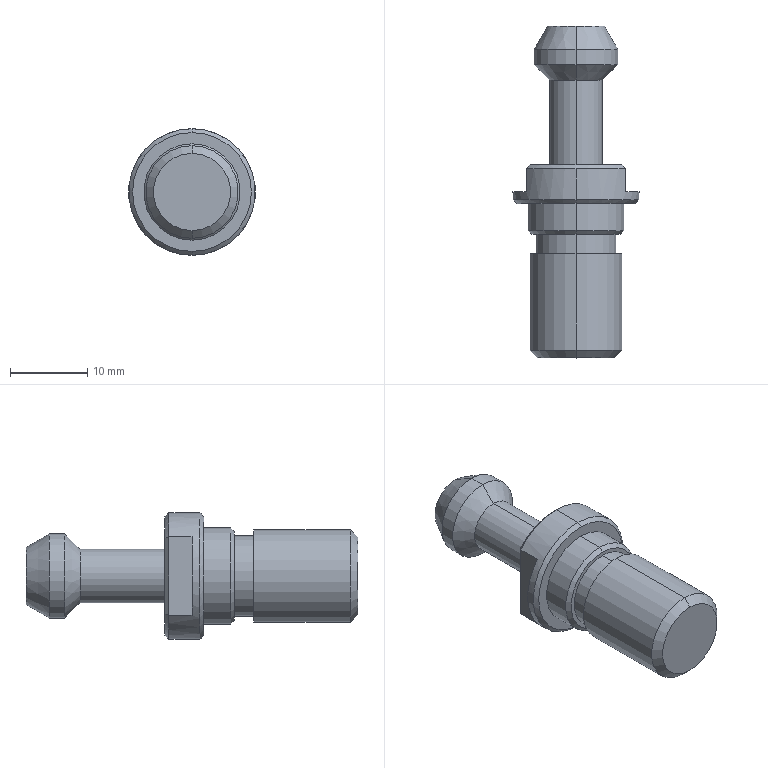Part | SolidWorks | features Chamfer 2, ICE 1, Revolution 1 | 1 solid | 37 faces | box 16.4 x 43 x 16.4 mm | volume 4091 mm3 | cone 13 | cylinder 12 | plane 12 | commonest cylinder face diameters 6.9 x2 10.4 x2 10.9 x2 12 x2 12.5 x2 16.4 x2
STEP:
#1=CARTESIAN_POINT('',(0.,16.,-5.75));
#2=VERTEX_POINT('',#1);
#3=CARTESIAN_POINT('',(0.,16.,5.75));
#4=VERTEX_POINT('',#3);
#5=CARTESIAN_POINT('',(0.,16.,0.));
#6=DIRECTION('',(0.,-1.,0.));
#7=DIRECTION('',(0.,0.,-1.));
#8=AXIS2_PLACEMENT_3D('',#5,#6,#7);
#9=CIRCLE('',#8,5.75);
#10=EDGE_CURVE('',#2,#4,#9,.T.);
#11=ORIENTED_EDGE('',*,*,#10,.F.);
#12=CARTESIAN_POINT('',(0.,16.5,-6.25));
#13=VERTEX_POINT('',#12);
#14=CARTESIAN_POINT('',(0.,16.,-5.75));
#15=DIRECTION('',(0.,0.7071,-0.7071));
#16=VECTOR('',#15,1000.);
#17=LINE('',#14,#16);
#18=EDGE_CURVE('',#2,#13,#17,.T.);
#19=ORIENTED_EDGE('',*,*,#18,.T.);
#20=CARTESIAN_POINT('',(0.,16.5,6.25));
#21=VERTEX_POINT('',#20);
#22=CARTESIAN_POINT('',(0.,16.5,0.));
#23=DIRECTION('',(0.,1.,0.));
#24=DIRECTION('',(0.,0.,-1.));
#25=AXIS2_PLACEMENT_3D('',#22,#23,#24);
#26=CIRCLE('',#25,6.25);
#27=EDGE_CURVE('',#21,#13,#26,.T.);
#28=ORIENTED_EDGE('',*,*,#27,.F.);
#29=CARTESIAN_POINT('',(0.,16.,5.75));
#30=DIRECTION('',(0.,0.7071,0.7071));
#31=VECTOR('',#30,1000.);
#32=LINE('',#29,#31);
#33=EDGE_CURVE('',#4,#21,#32,.T.);
#34=ORIENTED_EDGE('',*,*,#33,.F.);
#35=EDGE_LOOP('',(#11,#19,#28,#34));
#36=FACE_OUTER_BOUND('',#35,.T.);
#37=CARTESIAN_POINT('',(0.,16.,0.));
#38=DIRECTION('',(0.,1.,0.));
#39=DIRECTION('',(0.,0.,1.));
#40=AXIS2_PLACEMENT_3D('',#37,#38,#39);
#41=CONICAL_SURFACE('',#40,5.75,0.7854);
#42=ADVANCED_FACE('',(#36),#41,.T.);
#43=CARTESIAN_POINT('',(0.,20.,-7.7));
#44=VERTEX_POINT('',#43);
#45=CARTESIAN_POINT('',(0.,20.,7.7));
#46=VERTEX_POINT('',#45);
#47=CARTESIAN_POINT('',(0.,20.,0.));
#48=DIRECTION('',(0.,-1.,0.));
#49=DIRECTION('',(0.,0.,-1.));
#50=AXIS2_PLACEMENT_3D('',#47,#48,#49);
#51=CIRCLE('',#50,7.7);
#52=EDGE_CURVE('',#44,#46,#51,.T.);
#53=ORIENTED_EDGE('',*,*,#52,.F.);
#54=CARTESIAN_POINT('',(0.,20.5,-8.2));
#55=VERTEX_POINT('',#54);
#56=CARTESIAN_POINT('',(0.,20.,-7.7));
#57=DIRECTION('',(0.,0.7071,-0.7071));
#58=VECTOR('',#57,1000.);
#59=LINE('',#56,#58);
#60=EDGE_CURVE('',#44,#55,#59,.T.);
#61=ORIENTED_EDGE('',*,*,#60,.T.);
#62=CARTESIAN_POINT('',(0.,20.5,8.2));
#63=VERTEX_POINT('',#62);
#64=CARTESIAN_POINT('',(0.,20.5,0.));
#65=DIRECTION('',(0.,1.,0.));
#66=DIRECTION('',(0.,0.,-1.));
#67=AXIS2_PLACEMENT_3D('',#64,#65,#66);
#68=CIRCLE('',#67,8.2);
#69=EDGE_CURVE('',#63,#55,#68,.T.);
#70=ORIENTED_EDGE('',*,*,#69,.F.);
#71=CARTESIAN_POINT('',(0.,20.,7.7));
#72=DIRECTION('',(0.,0.7071,0.7071));
#73=VECTOR('',#72,1000.);
#74=LINE('',#71,#73);
#75=EDGE_CURVE('',#46,#63,#74,.T.);
#76=ORIENTED_EDGE('',*,*,#75,.F.);
#77=EDGE_LOOP('',(#53,#61,#70,#76));
#78=FACE_OUTER_BOUND('',#77,.T.);
#79=CARTESIAN_POINT('',(0.,20.,0.));
#80=DIRECTION('',(0.,1.,0.));
#81=DIRECTION('',(0.,0.,1.));
#82=AXIS2_PLACEMENT_3D('',#79,#80,#81);
#83=CONICAL_SURFACE('',#82,7.7,0.7854);
#84=ADVANCED_FACE('',(#78),#83,.T.);
#85=CARTESIAN_POINT('',(0.,25.,-7.7));
#86=VERTEX_POINT('',#85);
#87=CARTESIAN_POINT('',(-5.95,25.,-4.887));
#88=VERTEX_POINT('',#87);
#89=CARTESIAN_POINT('',(0.,25.,0.));
#90=DIRECTION('',(0.,1.,0.));
#91=DIRECTION('',(0.,0.,1.));
#92=AXIS2_PLACEMENT_3D('',#89,#90,#91);
#93=CIRCLE('',#92,7.7);
#94=EDGE_CURVE('',#86,#88,#93,.T.);
#95=ORIENTED_EDGE('',*,*,#94,.F.);
#96=CARTESIAN_POINT('',(0.,24.5,-8.2));
#97=VERTEX_POINT('',#96);
#98=CARTESIAN_POINT('',(0.,24.5,-8.2));
#99=DIRECTION('',(0.,-0.7071,-0.7071));
#100=VECTOR('',#99,1000.);
#101=LINE('',#98,#100);
#102=EDGE_CURVE('',#86,#97,#101,.T.);
#103=ORIENTED_EDGE('',*,*,#102,.T.);
#104=CARTESIAN_POINT('',(-6.45,24.5,-5.063));
#105=VERTEX_POINT('',#104);
#106=CARTESIAN_POINT('',(0.,24.5,0.));
#107=DIRECTION('',(0.,-1.,0.));
#108=DIRECTION('',(0.,0.,1.));
#109=AXIS2_PLACEMENT_3D('',#106,#107,#108);
#110=CIRCLE('',#109,8.2);
#111=EDGE_CURVE('',#105,#97,#110,.T.);
#112=ORIENTED_EDGE('',*,*,#111,.F.);
#113=CARTESIAN_POINT('',(-6.45,24.5,-5.063));
#114=CARTESIAN_POINT('',(-6.283,24.667,-5.006));
#115=CARTESIAN_POINT('',(-6.116,24.834,-4.947));
#116=CARTESIAN_POINT('',(-5.95,25.,-4.887));
#117=B_SPLINE_CURVE_WITH_KNOTS('',3,(#113,#114,#115,#116),.UNSPECIFIED.,.F.,.F.,(4,4),(0.,0.0007286),.UNSPECIFIED.);
#118=EDGE_CURVE('',#105,#88,#117,.T.);
#119=ORIENTED_EDGE('',*,*,#118,.T.);
#120=EDGE_LOOP('',(#95,#103,#112,#119));
#121=FACE_OUTER_BOUND('',#120,.T.);
#122=CARTESIAN_POINT('',(0.,24.5,0.));
#123=DIRECTION('',(0.,-1.,0.));
#124=DIRECTION('',(0.,0.,-1.));
#125=AXIS2_PLACEMENT_3D('',#122,#123,#124);
#126=CONICAL_SURFACE('',#125,8.2,0.7854);
#127=ADVANCED_FACE('',(#121),#126,.T.);
#128=CARTESIAN_POINT('',(0.,0.,-5.));
#129=VERTEX_POINT('',#128);
#130=CARTESIAN_POINT('',(0.,0.,5.));
#131=VERTEX_POINT('',#130);
#132=CARTESIAN_POINT('',(0.,0.,0.));
#133=DIRECTION('',(0.,-1.,0.));
#134=DIRECTION('',(0.,0.,-1.));
#135=AXIS2_PLACEMENT_3D('',#132,#133,#134);
#136=CIRCLE('',#135,5.);
#137=EDGE_CURVE('',#129,#131,#136,.T.);
#138=ORIENTED_EDGE('',*,*,#137,.F.);
#139=CARTESIAN_POINT('',(0.,1.,-6.));
#140=VERTEX_POINT('',#139);
#141=CARTESIAN_POINT('',(0.,0.,-5.));
#142=DIRECTION('',(0.,0.7071,-0.7071));
#143=VECTOR('',#142,1000.);
#144=LINE('',#141,#143);
#145=EDGE_CURVE('',#129,#140,#144,.T.);
#146=ORIENTED_EDGE('',*,*,#145,.T.);
#147=CARTESIAN_POINT('',(0.,1.,6.));
#148=VERTEX_POINT('',#147);
#149=CARTESIAN_POINT('',(0.,1.,0.));
#150=DIRECTION('',(0.,1.,0.));
#151=DIRECTION('',(0.,0.,-1.));
#152=AXIS2_PLACEMENT_3D('',#149,#150,#151);
#153=CIRCLE('',#152,6.);
#154=EDGE_CURVE('',#148,#140,#153,.T.);
#155=ORIENTED_EDGE('',*,*,#154,.F.);
#156=CARTESIAN_POINT('',(0.,0.,5.));
#157=DIRECTION('',(0.,0.7071,0.7071));
#158=VECTOR('',#157,1000.);
#159=LINE('',#156,#158);
#160=EDGE_CURVE('',#131,#148,#159,.T.);
#161=ORIENTED_EDGE('',*,*,#160,.F.);
#162=EDGE_LOOP('',(#138,#146,#155,#161));
#163=FACE_OUTER_BOUND('',#162,.T.);
#164=CARTESIAN_POINT('',(0.,0.,0.));
#165=DIRECTION('',(0.,1.,0.));
#166=DIRECTION('',(0.,0.,1.));
#167=AXIS2_PLACEMENT_3D('',#164,#165,#166);
#168=CONICAL_SURFACE('',#167,5.,0.7854);
#169=ADVANCED_FACE('',(#163),#168,.T.);
#170=CARTESIAN_POINT('',(0.,13.5,-6.));
#171=VERTEX_POINT('',#170);
#172=CARTESIAN_POINT('',(0.,13.5,6.));
#173=VERTEX_POINT('',#172);
#174=CARTESIAN_POINT('',(0.,13.5,0.));
#175=DIRECTION('',(0.,-1.,0.));
#176=DIRECTION('',(0.,0.,-1.));
#177=AXIS2_PLACEMENT_3D('',#174,#175,#176);
#178=CIRCLE('',#177,6.);
#179=EDGE_CURVE('',#171,#173,#178,.T.);
#180=ORIENTED_EDGE('',*,*,#179,.T.);
#181=CARTESIAN_POINT('',(0.,0.,6.));
#182=DIRECTION('',(0.,-1.,0.));
#183=VECTOR('',#182,1000.);
#184=LINE('',#181,#183);
#185=EDGE_CURVE('',#173,#148,#184,.T.);
#186=ORIENTED_EDGE('',*,*,#185,.T.);
#187=ORIENTED_EDGE('',*,*,#154,.T.);
#188=CARTESIAN_POINT('',(0.,0.,-6.));
#189=DIRECTION('',(0.,-1.,0.));
#190=VECTOR('',#189,1000.);
#191=LINE('',#188,#190);
#192=EDGE_CURVE('',#171,#140,#191,.T.);
#193=ORIENTED_EDGE('',*,*,#192,.F.);
#194=EDGE_LOOP('',(#180,#186,#187,#193));
#195=FACE_OUTER_BOUND('',#194,.T.);
#196=CARTESIAN_POINT('',(0.,0.,0.));
#197=DIRECTION('',(0.,-1.,0.));
#198=DIRECTION('',(0.,0.,-1.));
#199=AXIS2_PLACEMENT_3D('',#196,#197,#198);
#200=CYLINDRICAL_SURFACE('',#199,6.);
#201=ADVANCED_FACE('',(#195),#200,.T.);
#202=CARTESIAN_POINT('',(0.,16.,-5.2));
#203=VERTEX_POINT('',#202);
#204=CARTESIAN_POINT('',(0.,16.,5.2));
#205=VERTEX_POINT('',#204);
#206=CARTESIAN_POINT('',(0.,16.,0.));
#207=DIRECTION('',(0.,-1.,0.));
#208=DIRECTION('',(0.,0.,-1.));
#209=AXIS2_PLACEMENT_3D('',#206,#207,#208);
#210=CIRCLE('',#209,5.2);
#211=EDGE_CURVE('',#203,#205,#210,.T.);
#212=ORIENTED_EDGE('',*,*,#211,.T.);
#213=CARTESIAN_POINT('',(0.,13.5,5.2));
#214=VERTEX_POINT('',#213);
#215=CARTESIAN_POINT('',(0.,0.,5.2));
#216=DIRECTION('',(0.,-1.,0.));
#217=VECTOR('',#216,1000.);
#218=LINE('',#215,#217);
#219=EDGE_CURVE('',#205,#214,#218,.T.);
#220=ORIENTED_EDGE('',*,*,#219,.T.);
#221=CARTESIAN_POINT('',(0.,13.5,-5.2));
#222=VERTEX_POINT('',#221);
#223=CARTESIAN_POINT('',(0.,13.5,0.));
#224=DIRECTION('',(0.,-1.,0.));
#225=DIRECTION('',(0.,0.,-1.));
#226=AXIS2_PLACEMENT_3D('',#223,#224,#225);
#227=CIRCLE('',#226,5.2);
#228=EDGE_CURVE('',#222,#214,#227,.T.);
#229=ORIENTED_EDGE('',*,*,#228,.F.);
#230=CARTESIAN_POINT('',(0.,0.,-5.2));
#231=DIRECTION('',(0.,-1.,0.));
#232=VECTOR('',#231,1000.);
#233=LINE('',#230,#232);
#234=EDGE_CURVE('',#203,#222,#233,.T.);
#235=ORIENTED_EDGE('',*,*,#234,.F.);
#236=EDGE_LOOP('',(#212,#220,#229,#235));
#237=FACE_OUTER_BOUND('',#236,.T.);
#238=CARTESIAN_POINT('',(0.,0.,0.));
#239=DIRECTION('',(0.,-1.,0.));
#240=DIRECTION('',(0.,0.,-1.));
#241=AXIS2_PLACEMENT_3D('',#238,#239,#240);
#242=CYLINDRICAL_SURFACE('',#241,5.2);
#243=ADVANCED_FACE('',(#237),#242,.T.);
#244=CARTESIAN_POINT('',(0.,20.,-6.25));
#245=VERTEX_POINT('',#244);
#246=CARTESIAN_POINT('',(0.,20.,6.25));
#247=VERTEX_POINT('',#246);
#248=CARTESIAN_POINT('',(0.,20.,0.));
#249=DIRECTION('',(0.,-1.,0.));
#250=DIRECTION('',(0.,0.,-1.));
#251=AXIS2_PLACEMENT_3D('',#248,#249,#250);
#252=CIRCLE('',#251,6.25);
#253=EDGE_CURVE('',#245,#247,#252,.T.);
#254=ORIENTED_EDGE('',*,*,#253,.T.);
#255=CARTESIAN_POINT('',(0.,0.,6.25));
#256=DIRECTION('',(0.,-1.,0.));
#257=VECTOR('',#256,1000.);
#258=LINE('',#255,#257);
#259=EDGE_CURVE('',#247,#21,#258,.T.);
#260=ORIENTED_EDGE('',*,*,#259,.T.);
#261=ORIENTED_EDGE('',*,*,#27,.T.);
#262=CARTESIAN_POINT('',(0.,0.,-6.25));
#263=DIRECTION('',(0.,-1.,0.));
#264=VECTOR('',#263,1000.);
#265=LINE('',#262,#264);
#266=EDGE_CURVE('',#245,#13,#265,.T.);
#267=ORIENTED_EDGE('',*,*,#266,.F.);
#268=EDGE_LOOP('',(#254,#260,#261,#267));
#269=FACE_OUTER_BOUND('',#268,.T.);
#270=CARTESIAN_POINT('',(0.,0.,0.));
#271=DIRECTION('',(0.,-1.,0.));
#272=DIRECTION('',(0.,0.,-1.));
#273=AXIS2_PLACEMENT_3D('',#270,#271,#272);
#274=CYLINDRICAL_SURFACE('',#273,6.25);
#275=ADVANCED_FACE('',(#269),#274,.T.);
#276=CARTESIAN_POINT('',(6.45,24.5,5.063));
#277=VERTEX_POINT('',#276);
#278=CARTESIAN_POINT('',(0.,24.5,8.2));
#279=VERTEX_POINT('',#278);
#280=CARTESIAN_POINT('',(0.,24.5,0.));
#281=DIRECTION('',(0.,-1.,0.));
#282=DIRECTION('',(0.,0.,1.));
#283=AXIS2_PLACEMENT_3D('',#280,#281,#282);
#284=CIRCLE('',#283,8.2);
#285=EDGE_CURVE('',#277,#279,#284,.T.);
#286=ORIENTED_EDGE('',*,*,#285,.T.);
#287=CARTESIAN_POINT('',(0.,0.,8.2));
#288=DIRECTION('',(0.,-1.,0.));
#289=VECTOR('',#288,1000.);
#290=LINE('',#287,#289);
#291=EDGE_CURVE('',#279,#63,#290,.T.);
#292=ORIENTED_EDGE('',*,*,#291,.T.);
#293=ORIENTED_EDGE('',*,*,#69,.T.);
#294=CARTESIAN_POINT('',(0.,0.,-8.2));
#295=DIRECTION('',(0.,-1.,0.));
#296=VECTOR('',#295,1000.);
#297=LINE('',#294,#296);
#298=EDGE_CURVE('',#97,#55,#297,.T.);
#299=ORIENTED_EDGE('',*,*,#298,.F.);
#300=CARTESIAN_POINT('',(6.45,24.5,-5.063));
#301=VERTEX_POINT('',#300);
#302=CARTESIAN_POINT('',(0.,24.5,0.));
#303=DIRECTION('',(0.,-1.,0.));
#304=DIRECTION('',(0.,0.,1.));
#305=AXIS2_PLACEMENT_3D('',#302,#303,#304);
#306=CIRCLE('',#305,8.2);
#307=EDGE_CURVE('',#97,#301,#306,.T.);
#308=ORIENTED_EDGE('',*,*,#307,.T.);
#309=CARTESIAN_POINT('',(6.45,21.5,-5.063));
#310=VERTEX_POINT('',#309);
#311=CARTESIAN_POINT('',(6.45,0.,-5.063));
#312=DIRECTION('',(0.,1.,0.));
#313=VECTOR('',#312,1000.);
#314=LINE('',#311,#313);
#315=EDGE_CURVE('',#310,#301,#314,.T.);
#316=ORIENTED_EDGE('',*,*,#315,.F.);
#317=CARTESIAN_POINT('',(6.45,21.5,5.063));
#318=VERTEX_POINT('',#317);
#319=CARTESIAN_POINT('',(0.,21.5,0.));
#320=DIRECTION('',(0.,-1.,0.));
#321=DIRECTION('',(0.,0.,1.));
#322=AXIS2_PLACEMENT_3D('',#319,#320,#321);
#323=CIRCLE('',#322,8.2);
#324=EDGE_CURVE('',#310,#318,#323,.T.);
#325=ORIENTED_EDGE('',*,*,#324,.T.);
#326=CARTESIAN_POINT('',(6.45,0.,5.063));
#327=DIRECTION('',(0.,-1.,0.));
#328=VECTOR('',#327,1000.);
#329=LINE('',#326,#328);
#330=EDGE_CURVE('',#277,#318,#329,.T.);
#331=ORIENTED_EDGE('',*,*,#330,.F.);
#332=EDGE_LOOP('',(#286,#292,#293,#299,#308,#316,#325,#331));
#333=FACE_OUTER_BOUND('',#332,.T.);
#334=CARTESIAN_POINT('',(0.,0.,0.));
#335=DIRECTION('',(0.,-1.,0.));
#336=DIRECTION('',(0.,0.,-1.));
#337=AXIS2_PLACEMENT_3D('',#334,#335,#336);
#338=CYLINDRICAL_SURFACE('',#337,8.2);
#339=ADVANCED_FACE('',(#333),#338,.T.);
#340=CARTESIAN_POINT('',(0.,36.,-3.45));
#341=VERTEX_POINT('',#340);
#342=CARTESIAN_POINT('',(0.,36.,3.45));
#343=VERTEX_POINT('',#342);
#344=CARTESIAN_POINT('',(0.,36.,0.));
#345=DIRECTION('',(0.,-1.,0.));
#346=DIRECTION('',(0.,0.,-1.));
#347=AXIS2_PLACEMENT_3D('',#344,#345,#346);
#348=CIRCLE('',#347,3.45);
#349=EDGE_CURVE('',#341,#343,#348,.T.);
#350=ORIENTED_EDGE('',*,*,#349,.T.);
#351=CARTESIAN_POINT('',(0.,25.,3.45));
#352=VERTEX_POINT('',#351);
#353=CARTESIAN_POINT('',(0.,0.,3.45));
#354=DIRECTION('',(0.,-1.,0.));
#355=VECTOR('',#354,1000.);
#356=LINE('',#353,#355);
#357=EDGE_CURVE('',#343,#352,#356,.T.);
#358=ORIENTED_EDGE('',*,*,#357,.T.);
#359=CARTESIAN_POINT('',(0.,25.,-3.45));
#360=VERTEX_POINT('',#359);
#361=CARTESIAN_POINT('',(0.,25.,0.));
#362=DIRECTION('',(0.,-1.,0.));
#363=DIRECTION('',(0.,0.,-1.));
#364=AXIS2_PLACEMENT_3D('',#361,#362,#363);
#365=CIRCLE('',#364,3.45);
#366=EDGE_CURVE('',#360,#352,#365,.T.);
#367=ORIENTED_EDGE('',*,*,#366,.F.);
#368=CARTESIAN_POINT('',(0.,0.,-3.45));
#369=DIRECTION('',(0.,-1.,0.));
#370=VECTOR('',#369,1000.);
#371=LINE('',#368,#370);
#372=EDGE_CURVE('',#341,#360,#371,.T.);
#373=ORIENTED_EDGE('',*,*,#372,.F.);
#374=EDGE_LOOP('',(#350,#358,#367,#373));
#375=FACE_OUTER_BOUND('',#374,.T.);
#376=CARTESIAN_POINT('',(0.,0.,0.));
#377=DIRECTION('',(0.,-1.,0.));
#378=DIRECTION('',(0.,0.,-1.));
#379=AXIS2_PLACEMENT_3D('',#376,#377,#378);
#380=CYLINDRICAL_SURFACE('',#379,3.45);
#381=ADVANCED_FACE('',(#375),#380,.T.);
#382=ORIENTED_EDGE('',*,*,#349,.F.);
#383=CARTESIAN_POINT('',(0.,38.,-5.45));
#384=VERTEX_POINT('',#383);
#385=CARTESIAN_POINT('',(0.,36.,-3.45));
#386=DIRECTION('',(0.,0.7071,-0.7071));
#387=VECTOR('',#386,1000.);
#388=LINE('',#385,#387);
#389=EDGE_CURVE('',#341,#384,#388,.T.);
#390=ORIENTED_EDGE('',*,*,#389,.T.);
#391=CARTESIAN_POINT('',(0.,38.,5.45));
#392=VERTEX_POINT('',#391);
#393=CARTESIAN_POINT('',(0.,38.,0.));
#394=DIRECTION('',(0.,-1.,0.));
#395=DIRECTION('',(0.,0.,-1.));
#396=AXIS2_PLACEMENT_3D('',#393,#394,#395);
#397=CIRCLE('',#396,5.45);
#398=EDGE_CURVE('',#384,#392,#397,.T.);
#399=ORIENTED_EDGE('',*,*,#398,.T.);
#400=CARTESIAN_POINT('',(0.,36.,3.45));
#401=DIRECTION('',(0.,0.7071,0.7071));
#402=VECTOR('',#401,1000.);
#403=LINE('',#400,#402);
#404=EDGE_CURVE('',#343,#392,#403,.T.);
#405=ORIENTED_EDGE('',*,*,#404,.F.);
#406=EDGE_LOOP('',(#382,#390,#399,#405));
#407=FACE_OUTER_BOUND('',#406,.T.);
#408=CARTESIAN_POINT('',(0.,36.,0.));
#409=DIRECTION('',(0.,1.,0.));
#410=DIRECTION('',(0.,0.,1.));
#411=AXIS2_PLACEMENT_3D('',#408,#409,#410);
#412=CONICAL_SURFACE('',#411,3.45,0.7854);
#413=ADVANCED_FACE('',(#407),#412,.T.);
#414=CARTESIAN_POINT('',(0.,40.,-5.45));
#415=VERTEX_POINT('',#414);
#416=CARTESIAN_POINT('',(0.,40.,5.45));
#417=VERTEX_POINT('',#416);
#418=CARTESIAN_POINT('',(0.,40.,0.));
#419=DIRECTION('',(0.,-1.,0.));
#420=DIRECTION('',(0.,0.,-1.));
#421=AXIS2_PLACEMENT_3D('',#418,#419,#420);
#422=CIRCLE('',#421,5.45);
#423=EDGE_CURVE('',#415,#417,#422,.T.);
#424=ORIENTED_EDGE('',*,*,#423,.T.);
#425=CARTESIAN_POINT('',(0.,0.,5.45));
#426=DIRECTION('',(0.,-1.,0.));
#427=VECTOR('',#426,1000.);
#428=LINE('',#425,#427);
#429=EDGE_CURVE('',#417,#392,#428,.T.);
#430=ORIENTED_EDGE('',*,*,#429,.T.);
#431=ORIENTED_EDGE('',*,*,#398,.F.);
#432=CARTESIAN_POINT('',(0.,0.,-5.45));
#433=DIRECTION('',(0.,-1.,0.));
#434=VECTOR('',#433,1000.);
#435=LINE('',#432,#434);
#436=EDGE_CURVE('',#415,#384,#435,.T.);
#437=ORIENTED_EDGE('',*,*,#436,.F.);
#438=EDGE_LOOP('',(#424,#430,#431,#437));
#439=FACE_OUTER_BOUND('',#438,.T.);
#440=CARTESIAN_POINT('',(0.,0.,0.));
#441=DIRECTION('',(0.,-1.,0.));
#442=DIRECTION('',(0.,0.,-1.));
#443=AXIS2_PLACEMENT_3D('',#440,#441,#442);
#444=CYLINDRICAL_SURFACE('',#443,5.45);
#445=ADVANCED_FACE('',(#439),#444,.T.);
#446=CARTESIAN_POINT('',(0.,43.,-3.718));
#447=VERTEX_POINT('',#446);
#448=CARTESIAN_POINT('',(0.,43.,3.718));
#449=VERTEX_POINT('',#448);
#450=CARTESIAN_POINT('',(0.,43.,0.));
#451=DIRECTION('',(0.,-1.,0.));
#452=DIRECTION('',(0.,0.,-1.));
#453=AXIS2_PLACEMENT_3D('',#450,#451,#452);
#454=CIRCLE('',#453,3.718);
#455=EDGE_CURVE('',#447,#449,#454,.T.);
#456=ORIENTED_EDGE('',*,*,#455,.T.);
#457=CARTESIAN_POINT('',(0.,40.,5.45));
#458=DIRECTION('',(0.,-0.866,0.5));
#459=VECTOR('',#458,1000.);
#460=LINE('',#457,#459);
#461=EDGE_CURVE('',#449,#417,#460,.T.);
#462=ORIENTED_EDGE('',*,*,#461,.T.);
#463=ORIENTED_EDGE('',*,*,#423,.F.);
#464=CARTESIAN_POINT('',(0.,40.,-5.45));
#465=DIRECTION('',(0.,-0.866,-0.5));
#466=VECTOR('',#465,1000.);
#467=LINE('',#464,#466);
#468=EDGE_CURVE('',#447,#415,#467,.T.);
#469=ORIENTED_EDGE('',*,*,#468,.F.);
#470=EDGE_LOOP('',(#456,#462,#463,#469));
#471=FACE_OUTER_BOUND('',#470,.T.);
#472=CARTESIAN_POINT('',(0.,40.,0.));
#473=DIRECTION('',(0.,-1.,0.));
#474=DIRECTION('',(0.,0.,-1.));
#475=AXIS2_PLACEMENT_3D('',#472,#473,#474);
#476=CONICAL_SURFACE('',#475,5.45,0.5236);
#477=ADVANCED_FACE('',(#471),#476,.T.);
#478=ORIENTED_EDGE('',*,*,#455,.F.);
#479=CARTESIAN_POINT('',(0.,43.,0.));
#480=DIRECTION('',(0.,-1.,0.));
#481=DIRECTION('',(0.,0.,-1.));
#482=AXIS2_PLACEMENT_3D('',#479,#480,#481);
#483=CIRCLE('',#482,3.718);
#484=EDGE_CURVE('',#449,#447,#483,.T.);
#485=ORIENTED_EDGE('',*,*,#484,.F.);
#486=EDGE_LOOP('',(#478,#485));
#487=FACE_OUTER_BOUND('',#486,.T.);
#488=CARTESIAN_POINT('',(0.,43.,0.));
#489=DIRECTION('',(0.,1.,0.));
#490=DIRECTION('',(0.,0.,1.));
#491=AXIS2_PLACEMENT_3D('',#488,#489,#490);
#492=PLANE('',#491);
#493=ADVANCED_FACE('',(#487),#492,.T.);
#494=ORIENTED_EDGE('',*,*,#461,.F.);
#495=ORIENTED_EDGE('',*,*,#484,.T.);
#496=ORIENTED_EDGE('',*,*,#468,.T.);
#497=CARTESIAN_POINT('',(0.,40.,0.));
#498=DIRECTION('',(0.,-1.,0.));
#499=DIRECTION('',(0.,0.,-1.));
#500=AXIS2_PLACEMENT_3D('',#497,#498,#499);
#501=CIRCLE('',#500,5.45);
#502=EDGE_CURVE('',#417,#415,#501,.T.);
#503=ORIENTED_EDGE('',*,*,#502,.F.);
#504=EDGE_LOOP('',(#494,#495,#496,#503));
#505=FACE_OUTER_BOUND('',#504,.T.);
#506=CARTESIAN_POINT('',(0.,40.,0.));
#507=DIRECTION('',(0.,-1.,0.));
#508=DIRECTION('',(0.,0.,-1.));
#509=AXIS2_PLACEMENT_3D('',#506,#507,#508);
#510=CONICAL_SURFACE('',#509,5.45,0.5236);
#511=ADVANCED_FACE('',(#505),#510,.T.);
#512=ORIENTED_EDGE('',*,*,#429,.F.);
#513=ORIENTED_EDGE('',*,*,#502,.T.);
#514=ORIENTED_EDGE('',*,*,#436,.T.);
#515=CARTESIAN_POINT('',(0.,38.,0.));
#516=DIRECTION('',(0.,-1.,0.));
#517=DIRECTION('',(0.,0.,-1.));
#518=AXIS2_PLACEMENT_3D('',#515,#516,#517);
#519=CIRCLE('',#518,5.45);
#520=EDGE_CURVE('',#392,#384,#519,.T.);
#521=ORIENTED_EDGE('',*,*,#520,.F.);
#522=EDGE_LOOP('',(#512,#513,#514,#521));
#523=FACE_OUTER_BOUND('',#522,.T.);
#524=CARTESIAN_POINT('',(0.,0.,0.));
#525=DIRECTION('',(0.,-1.,0.));
#526=DIRECTION('',(0.,0.,-1.));
#527=AXIS2_PLACEMENT_3D('',#524,#525,#526);
#528=CYLINDRICAL_SURFACE('',#527,5.45);
#529=ADVANCED_FACE('',(#523),#528,.T.);
#530=ORIENTED_EDGE('',*,*,#389,.F.);
#531=CARTESIAN_POINT('',(0.,36.,0.));
#532=DIRECTION('',(0.,-1.,0.));
#533=DIRECTION('',(0.,0.,-1.));
#534=AXIS2_PLACEMENT_3D('',#531,#532,#533);
#535=CIRCLE('',#534,3.45);
#536=EDGE_CURVE('',#343,#341,#535,.T.);
#537=ORIENTED_EDGE('',*,*,#536,.F.);
#538=ORIENTED_EDGE('',*,*,#404,.T.);
#539=ORIENTED_EDGE('',*,*,#520,.T.);
#540=EDGE_LOOP('',(#530,#537,#538,#539));
#541=FACE_OUTER_BOUND('',#540,.T.);
#542=CARTESIAN_POINT('',(0.,36.,0.));
#543=DIRECTION('',(0.,1.,0.));
#544=DIRECTION('',(0.,0.,1.));
#545=AXIS2_PLACEMENT_3D('',#542,#543,#544);
#546=CONICAL_SURFACE('',#545,3.45,0.7854);
#547=ADVANCED_FACE('',(#541),#546,.T.);
#548=ORIENTED_EDGE('',*,*,#357,.F.);
#549=ORIENTED_EDGE('',*,*,#536,.T.);
#550=ORIENTED_EDGE('',*,*,#372,.T.);
#551=CARTESIAN_POINT('',(0.,25.,0.));
#552=DIRECTION('',(0.,-1.,0.));
#553=DIRECTION('',(0.,0.,-1.));
#554=AXIS2_PLACEMENT_3D('',#551,#552,#553);
#555=CIRCLE('',#554,3.45);
#556=EDGE_CURVE('',#352,#360,#555,.T.);
#557=ORIENTED_EDGE('',*,*,#556,.F.);
#558=EDGE_LOOP('',(#548,#549,#550,#557));
#559=FACE_OUTER_BOUND('',#558,.T.);
#560=CARTESIAN_POINT('',(0.,0.,0.));
#561=DIRECTION('',(0.,-1.,0.));
#562=DIRECTION('',(0.,0.,-1.));
#563=AXIS2_PLACEMENT_3D('',#560,#561,#562);
#564=CYLINDRICAL_SURFACE('',#563,3.45);
#565=ADVANCED_FACE('',(#559),#564,.T.);
#566=CARTESIAN_POINT('',(-5.95,25.,4.887));
#567=VERTEX_POINT('',#566);
#568=CARTESIAN_POINT('',(5.95,25.,4.887));
#569=VERTEX_POINT('',#568);
#570=CARTESIAN_POINT('',(0.,25.,0.));
#571=DIRECTION('',(0.,1.,0.));
#572=DIRECTION('',(0.,0.,1.));
#573=AXIS2_PLACEMENT_3D('',#570,#571,#572);
#574=CIRCLE('',#573,7.7);
#575=EDGE_CURVE('',#567,#569,#574,.T.);
#576=ORIENTED_EDGE('',*,*,#575,.T.);
#577=CARTESIAN_POINT('',(5.95,25.,-4.887));
#578=VERTEX_POINT('',#577);
#579=CARTESIAN_POINT('',(5.95,25.,-5.063));
#580=DIRECTION('',(0.,0.,-1.));
#581=VECTOR('',#580,1000.);
#582=LINE('',#579,#581);
#583=EDGE_CURVE('',#569,#578,#582,.T.);
#584=ORIENTED_EDGE('',*,*,#583,.T.);
#585=CARTESIAN_POINT('',(0.,25.,0.));
#586=DIRECTION('',(0.,1.,0.));
#587=DIRECTION('',(0.,0.,1.));
#588=AXIS2_PLACEMENT_3D('',#585,#586,#587);
#589=CIRCLE('',#588,7.7);
#590=EDGE_CURVE('',#578,#86,#589,.T.);
#591=ORIENTED_EDGE('',*,*,#590,.T.);
#592=ORIENTED_EDGE('',*,*,#94,.T.);
#593=CARTESIAN_POINT('',(-5.95,25.,5.063));
#594=DIRECTION('',(0.,0.,1.));
#595=VECTOR('',#594,1000.);
#596=LINE('',#593,#595);
#597=EDGE_CURVE('',#88,#567,#596,.T.);
#598=ORIENTED_EDGE('',*,*,#597,.T.);
#599=EDGE_LOOP('',(#576,#584,#591,#592,#598));
#600=FACE_OUTER_BOUND('',#599,.T.);
#601=ORIENTED_EDGE('',*,*,#366,.T.);
#602=ORIENTED_EDGE('',*,*,#556,.T.);
#603=EDGE_LOOP('',(#601,#602));
#604=FACE_BOUND('',#603,.T.);
#605=CARTESIAN_POINT('',(3.45,25.,0.));
#606=DIRECTION('',(0.,1.,0.));
#607=DIRECTION('',(0.,0.,1.));
#608=AXIS2_PLACEMENT_3D('',#605,#606,#607);
#609=PLANE('',#608);
#610=ADVANCED_FACE('',(#600,#604),#609,.T.);
#611=ORIENTED_EDGE('',*,*,#291,.F.);
#612=CARTESIAN_POINT('',(-6.45,24.5,5.063));
#613=VERTEX_POINT('',#612);
#614=CARTESIAN_POINT('',(0.,24.5,0.));
#615=DIRECTION('',(0.,-1.,0.));
#616=DIRECTION('',(0.,0.,1.));
#617=AXIS2_PLACEMENT_3D('',#614,#615,#616);
#618=CIRCLE('',#617,8.2);
#619=EDGE_CURVE('',#279,#613,#618,.T.);
#620=ORIENTED_EDGE('',*,*,#619,.T.);
#621=CARTESIAN_POINT('',(-6.45,21.5,5.063));
#622=VERTEX_POINT('',#621);
#623=CARTESIAN_POINT('',(-6.45,0.,5.063));
#624=DIRECTION('',(0.,1.,0.));
#625=VECTOR('',#624,1000.);
#626=LINE('',#623,#625);
#627=EDGE_CURVE('',#622,#613,#626,.T.);
#628=ORIENTED_EDGE('',*,*,#627,.F.);
#629=CARTESIAN_POINT('',(-6.45,21.5,-5.063));
#630=VERTEX_POINT('',#629);
#631=CARTESIAN_POINT('',(0.,21.5,0.));
#632=DIRECTION('',(0.,1.,0.));
#633=DIRECTION('',(0.,0.,-1.));
#634=AXIS2_PLACEMENT_3D('',#631,#632,#633);
#635=CIRCLE('',#634,8.2);
#636=EDGE_CURVE('',#630,#622,#635,.T.);
#637=ORIENTED_EDGE('',*,*,#636,.F.);
#638=CARTESIAN_POINT('',(-6.45,0.,-5.063));
#639=DIRECTION('',(0.,-1.,0.));
#640=VECTOR('',#639,1000.);
#641=LINE('',#638,#640);
#642=EDGE_CURVE('',#105,#630,#641,.T.);
#643=ORIENTED_EDGE('',*,*,#642,.F.);
#644=ORIENTED_EDGE('',*,*,#111,.T.);
#645=ORIENTED_EDGE('',*,*,#298,.T.);
#646=CARTESIAN_POINT('',(0.,20.5,0.));
#647=DIRECTION('',(0.,1.,0.));
#648=DIRECTION('',(0.,0.,-1.));
#649=AXIS2_PLACEMENT_3D('',#646,#647,#648);
#650=CIRCLE('',#649,8.2);
#651=EDGE_CURVE('',#55,#63,#650,.T.);
#652=ORIENTED_EDGE('',*,*,#651,.T.);
#653=EDGE_LOOP('',(#611,#620,#628,#637,#643,#644,#645,#652));
#654=FACE_OUTER_BOUND('',#653,.T.);
#655=CARTESIAN_POINT('',(0.,0.,0.));
#656=DIRECTION('',(0.,-1.,0.));
#657=DIRECTION('',(0.,0.,-1.));
#658=AXIS2_PLACEMENT_3D('',#655,#656,#657);
#659=CYLINDRICAL_SURFACE('',#658,8.2);
#660=ADVANCED_FACE('',(#654),#659,.T.);
#661=CARTESIAN_POINT('',(0.,20.,0.));
#662=DIRECTION('',(0.,-1.,0.));
#663=DIRECTION('',(0.,0.,-1.));
#664=AXIS2_PLACEMENT_3D('',#661,#662,#663);
#665=CIRCLE('',#664,7.7);
#666=EDGE_CURVE('',#46,#44,#665,.T.);
#667=ORIENTED_EDGE('',*,*,#666,.T.);
#668=ORIENTED_EDGE('',*,*,#52,.T.);
#669=EDGE_LOOP('',(#667,#668));
#670=FACE_OUTER_BOUND('',#669,.T.);
#671=ORIENTED_EDGE('',*,*,#253,.F.);
#672=CARTESIAN_POINT('',(0.,20.,0.));
#673=DIRECTION('',(0.,-1.,0.));
#674=DIRECTION('',(0.,0.,-1.));
#675=AXIS2_PLACEMENT_3D('',#672,#673,#674);
#676=CIRCLE('',#675,6.25);
#677=EDGE_CURVE('',#247,#245,#676,.T.);
#678=ORIENTED_EDGE('',*,*,#677,.F.);
#679=EDGE_LOOP('',(#671,#678));
#680=FACE_BOUND('',#679,.T.);
#681=CARTESIAN_POINT('',(8.2,20.,0.));
#682=DIRECTION('',(0.,-1.,0.));
#683=DIRECTION('',(0.,0.,-1.));
#684=AXIS2_PLACEMENT_3D('',#681,#682,#683);
#685=PLANE('',#684);
#686=ADVANCED_FACE('',(#670,#680),#685,.T.);
#687=ORIENTED_EDGE('',*,*,#259,.F.);
#688=ORIENTED_EDGE('',*,*,#677,.T.);
#689=ORIENTED_EDGE('',*,*,#266,.T.);
#690=CARTESIAN_POINT('',(0.,16.5,0.));
#691=DIRECTION('',(0.,1.,0.));
#692=DIRECTION('',(0.,0.,-1.));
#693=AXIS2_PLACEMENT_3D('',#690,#691,#692);
#694=CIRCLE('',#693,6.25);
#695=EDGE_CURVE('',#13,#21,#694,.T.);
#696=ORIENTED_EDGE('',*,*,#695,.T.);
#697=EDGE_LOOP('',(#687,#688,#689,#696));
#698=FACE_OUTER_BOUND('',#697,.T.);
#699=CARTESIAN_POINT('',(0.,0.,0.));
#700=DIRECTION('',(0.,-1.,0.));
#701=DIRECTION('',(0.,0.,-1.));
#702=AXIS2_PLACEMENT_3D('',#699,#700,#701);
#703=CYLINDRICAL_SURFACE('',#702,6.25);
#704=ADVANCED_FACE('',(#698),#703,.T.);
#705=CARTESIAN_POINT('',(0.,16.,0.));
#706=DIRECTION('',(0.,-1.,0.));
#707=DIRECTION('',(0.,0.,-1.));
#708=AXIS2_PLACEMENT_3D('',#705,#706,#707);
#709=CIRCLE('',#708,5.75);
#710=EDGE_CURVE('',#4,#2,#709,.T.);
#711=ORIENTED_EDGE('',*,*,#710,.T.);
#712=ORIENTED_EDGE('',*,*,#10,.T.);
#713=EDGE_LOOP('',(#711,#712));
#714=FACE_OUTER_BOUND('',#713,.T.);
#715=ORIENTED_EDGE('',*,*,#211,.F.);
#716=CARTESIAN_POINT('',(0.,16.,0.));
#717=DIRECTION('',(0.,-1.,0.));
#718=DIRECTION('',(0.,0.,-1.));
#719=AXIS2_PLACEMENT_3D('',#716,#717,#718);
#720=CIRCLE('',#719,5.2);
#721=EDGE_CURVE('',#205,#203,#720,.T.);
#722=ORIENTED_EDGE('',*,*,#721,.F.);
#723=EDGE_LOOP('',(#715,#722));
#724=FACE_BOUND('',#723,.T.);
#725=CARTESIAN_POINT('',(6.25,16.,0.));
#726=DIRECTION('',(0.,-1.,0.));
#727=DIRECTION('',(0.,0.,-1.));
#728=AXIS2_PLACEMENT_3D('',#725,#726,#727);
#729=PLANE('',#728);
#730=ADVANCED_FACE('',(#714,#724),#729,.T.);
#731=ORIENTED_EDGE('',*,*,#219,.F.);
#732=ORIENTED_EDGE('',*,*,#721,.T.);
#733=ORIENTED_EDGE('',*,*,#234,.T.);
#734=CARTESIAN_POINT('',(0.,13.5,0.));
#735=DIRECTION('',(0.,-1.,0.));
#736=DIRECTION('',(0.,0.,-1.));
#737=AXIS2_PLACEMENT_3D('',#734,#735,#736);
#738=CIRCLE('',#737,5.2);
#739=EDGE_CURVE('',#214,#222,#738,.T.);
#740=ORIENTED_EDGE('',*,*,#739,.F.);
#741=EDGE_LOOP('',(#731,#732,#733,#740));
#742=FACE_OUTER_BOUND('',#741,.T.);
#743=CARTESIAN_POINT('',(0.,0.,0.));
#744=DIRECTION('',(0.,-1.,0.));
#745=DIRECTION('',(0.,0.,-1.));
#746=AXIS2_PLACEMENT_3D('',#743,#744,#745);
#747=CYLINDRICAL_SURFACE('',#746,5.2);
#748=ADVANCED_FACE('',(#742),#747,.T.);
#749=ORIENTED_EDGE('',*,*,#228,.T.);
#750=ORIENTED_EDGE('',*,*,#739,.T.);
#751=EDGE_LOOP('',(#749,#750));
#752=FACE_BOUND('',#751,.T.);
#753=ORIENTED_EDGE('',*,*,#179,.F.);
#754=CARTESIAN_POINT('',(0.,13.5,0.));
#755=DIRECTION('',(0.,-1.,0.));
#756=DIRECTION('',(0.,0.,-1.));
#757=AXIS2_PLACEMENT_3D('',#754,#755,#756);
#758=CIRCLE('',#757,6.);
#759=EDGE_CURVE('',#173,#171,#758,.T.);
#760=ORIENTED_EDGE('',*,*,#759,.F.);
#761=EDGE_LOOP('',(#753,#760));
#762=FACE_OUTER_BOUND('',#761,.T.);
#763=CARTESIAN_POINT('',(5.2,13.5,0.));
#764=DIRECTION('',(0.,1.,0.));
#765=DIRECTION('',(0.,0.,1.));
#766=AXIS2_PLACEMENT_3D('',#763,#764,#765);
#767=PLANE('',#766);
#768=ADVANCED_FACE('',(#752,#762),#767,.T.);
#769=ORIENTED_EDGE('',*,*,#185,.F.);
#770=ORIENTED_EDGE('',*,*,#759,.T.);
#771=ORIENTED_EDGE('',*,*,#192,.T.);
#772=CARTESIAN_POINT('',(0.,1.,0.));
#773=DIRECTION('',(0.,1.,0.));
#774=DIRECTION('',(0.,0.,-1.));
#775=AXIS2_PLACEMENT_3D('',#772,#773,#774);
#776=CIRCLE('',#775,6.);
#777=EDGE_CURVE('',#140,#148,#776,.T.);
#778=ORIENTED_EDGE('',*,*,#777,.T.);
#779=EDGE_LOOP('',(#769,#770,#771,#778));
#780=FACE_OUTER_BOUND('',#779,.T.);
#781=CARTESIAN_POINT('',(0.,0.,0.));
#782=DIRECTION('',(0.,-1.,0.));
#783=DIRECTION('',(0.,0.,-1.));
#784=AXIS2_PLACEMENT_3D('',#781,#782,#783);
#785=CYLINDRICAL_SURFACE('',#784,6.);
#786=ADVANCED_FACE('',(#780),#785,.T.);
#787=CARTESIAN_POINT('',(0.,0.,0.));
#788=DIRECTION('',(0.,-1.,0.));
#789=DIRECTION('',(0.,0.,-1.));
#790=AXIS2_PLACEMENT_3D('',#787,#788,#789);
#791=CIRCLE('',#790,5.);
#792=EDGE_CURVE('',#131,#129,#791,.T.);
#793=ORIENTED_EDGE('',*,*,#792,.T.);
#794=ORIENTED_EDGE('',*,*,#137,.T.);
#795=EDGE_LOOP('',(#793,#794));
#796=FACE_OUTER_BOUND('',#795,.T.);
#797=CARTESIAN_POINT('',(6.,0.,0.));
#798=DIRECTION('',(0.,-1.,0.));
#799=DIRECTION('',(0.,0.,-1.));
#800=AXIS2_PLACEMENT_3D('',#797,#798,#799);
#801=PLANE('',#800);
#802=ADVANCED_FACE('',(#796),#801,.T.);
#803=ORIENTED_EDGE('',*,*,#145,.F.);
#804=ORIENTED_EDGE('',*,*,#792,.F.);
#805=ORIENTED_EDGE('',*,*,#160,.T.);
#806=ORIENTED_EDGE('',*,*,#777,.F.);
#807=EDGE_LOOP('',(#803,#804,#805,#806));
#808=FACE_OUTER_BOUND('',#807,.T.);
#809=CARTESIAN_POINT('',(0.,0.,0.));
#810=DIRECTION('',(0.,1.,0.));
#811=DIRECTION('',(0.,0.,1.));
#812=AXIS2_PLACEMENT_3D('',#809,#810,#811);
#813=CONICAL_SURFACE('',#812,5.,0.7854);
#814=ADVANCED_FACE('',(#808),#813,.T.);
#815=ORIENTED_EDGE('',*,*,#315,.T.);
#816=CARTESIAN_POINT('',(6.45,24.5,5.063));
#817=DIRECTION('',(0.,0.,1.));
#818=VECTOR('',#817,1000.);
#819=LINE('',#816,#818);
#820=EDGE_CURVE('',#301,#277,#819,.T.);
#821=ORIENTED_EDGE('',*,*,#820,.T.);
#822=ORIENTED_EDGE('',*,*,#330,.T.);
#823=CARTESIAN_POINT('',(6.45,21.5,-7.08));
#824=DIRECTION('',(0.,0.,1.));
#825=VECTOR('',#824,1000.);
#826=LINE('',#823,#825);
#827=EDGE_CURVE('',#310,#318,#826,.T.);
#828=ORIENTED_EDGE('',*,*,#827,.F.);
#829=EDGE_LOOP('',(#815,#821,#822,#828));
#830=FACE_OUTER_BOUND('',#829,.T.);
#831=CARTESIAN_POINT('',(6.45,21.5,-7.08));
#832=DIRECTION('',(-1.,0.,0.));
#833=DIRECTION('',(0.,0.,1.));
#834=AXIS2_PLACEMENT_3D('',#831,#832,#833);
#835=PLANE('',#834);
#836=ADVANCED_FACE('',(#830),#835,.F.);
#837=ORIENTED_EDGE('',*,*,#827,.T.);
#838=ORIENTED_EDGE('',*,*,#324,.F.);
#839=EDGE_LOOP('',(#837,#838));
#840=FACE_OUTER_BOUND('',#839,.T.);
#841=CARTESIAN_POINT('',(0.,21.5,0.));
#842=DIRECTION('',(0.,1.,0.));
#843=DIRECTION('',(0.,0.,1.));
#844=AXIS2_PLACEMENT_3D('',#841,#842,#843);
#845=PLANE('',#844);
#846=ADVANCED_FACE('',(#840),#845,.T.);
#847=ORIENTED_EDGE('',*,*,#627,.T.);
#848=CARTESIAN_POINT('',(-6.45,24.5,-5.063));
#849=DIRECTION('',(0.,0.,-1.));
#850=VECTOR('',#849,1000.);
#851=LINE('',#848,#850);
#852=EDGE_CURVE('',#613,#105,#851,.T.);
#853=ORIENTED_EDGE('',*,*,#852,.T.);
#854=ORIENTED_EDGE('',*,*,#642,.T.);
#855=CARTESIAN_POINT('',(-6.45,21.5,-7.08));
#856=DIRECTION('',(0.,0.,-1.));
#857=VECTOR('',#856,1000.);
#858=LINE('',#855,#857);
#859=EDGE_CURVE('',#622,#630,#858,.T.);
#860=ORIENTED_EDGE('',*,*,#859,.F.);
#861=EDGE_LOOP('',(#847,#853,#854,#860));
#862=FACE_OUTER_BOUND('',#861,.T.);
#863=CARTESIAN_POINT('',(-6.45,21.5,-7.08));
#864=DIRECTION('',(1.,0.,0.));
#865=DIRECTION('',(0.,0.,-1.));
#866=AXIS2_PLACEMENT_3D('',#863,#864,#865);
#867=PLANE('',#866);
#868=ADVANCED_FACE('',(#862),#867,.F.);
#869=ORIENTED_EDGE('',*,*,#636,.T.);
#870=ORIENTED_EDGE('',*,*,#859,.T.);
#871=EDGE_LOOP('',(#869,#870));
#872=FACE_OUTER_BOUND('',#871,.T.);
#873=CARTESIAN_POINT('',(0.,21.5,0.));
#874=DIRECTION('',(0.,-1.,0.));
#875=DIRECTION('',(0.,0.,-1.));
#876=AXIS2_PLACEMENT_3D('',#873,#874,#875);
#877=PLANE('',#876);
#878=ADVANCED_FACE('',(#872),#877,.F.);
#879=CARTESIAN_POINT('',(-5.95,25.,4.887));
#880=CARTESIAN_POINT('',(-6.116,24.834,4.947));
#881=CARTESIAN_POINT('',(-6.283,24.667,5.006));
#882=CARTESIAN_POINT('',(-6.45,24.5,5.063));
#883=B_SPLINE_CURVE_WITH_KNOTS('',3,(#879,#880,#881,#882),.UNSPECIFIED.,.F.,.F.,(4,4),(0.,0.0007286),.UNSPECIFIED.);
#884=EDGE_CURVE('',#567,#613,#883,.T.);
#885=ORIENTED_EDGE('',*,*,#884,.F.);
#886=ORIENTED_EDGE('',*,*,#597,.F.);
#887=ORIENTED_EDGE('',*,*,#118,.F.);
#888=ORIENTED_EDGE('',*,*,#852,.F.);
#889=EDGE_LOOP('',(#885,#886,#887,#888));
#890=FACE_OUTER_BOUND('',#889,.T.);
#891=CARTESIAN_POINT('',(-6.45,24.5,-7.08));
#892=DIRECTION('',(-0.7071,0.7071,0.));
#893=DIRECTION('',(0.,0.,1.));
#894=AXIS2_PLACEMENT_3D('',#891,#892,#893);
#895=PLANE('',#894);
#896=ADVANCED_FACE('',(#890),#895,.T.);
#897=ORIENTED_EDGE('',*,*,#102,.F.);
#898=ORIENTED_EDGE('',*,*,#590,.F.);
#899=CARTESIAN_POINT('',(6.45,24.5,-5.063));
#900=CARTESIAN_POINT('',(6.283,24.667,-5.006));
#901=CARTESIAN_POINT('',(6.116,24.834,-4.947));
#902=CARTESIAN_POINT('',(5.95,25.,-4.887));
#903=B_SPLINE_CURVE_WITH_KNOTS('',3,(#899,#900,#901,#902),.UNSPECIFIED.,.F.,.F.,(4,4),(0.,0.0007286),.UNSPECIFIED.);
#904=EDGE_CURVE('',#301,#578,#903,.T.);
#905=ORIENTED_EDGE('',*,*,#904,.F.);
#906=ORIENTED_EDGE('',*,*,#307,.F.);
#907=EDGE_LOOP('',(#897,#898,#905,#906));
#908=FACE_OUTER_BOUND('',#907,.T.);
#909=CARTESIAN_POINT('',(0.,24.5,0.));
#910=DIRECTION('',(0.,-1.,0.));
#911=DIRECTION('',(0.,0.,-1.));
#912=AXIS2_PLACEMENT_3D('',#909,#910,#911);
#913=CONICAL_SURFACE('',#912,8.2,0.7854);
#914=ADVANCED_FACE('',(#908),#913,.T.);
#915=ORIENTED_EDGE('',*,*,#884,.T.);
#916=ORIENTED_EDGE('',*,*,#619,.F.);
#917=ORIENTED_EDGE('',*,*,#285,.F.);
#918=CARTESIAN_POINT('',(5.95,25.,4.887));
#919=CARTESIAN_POINT('',(6.116,24.834,4.947));
#920=CARTESIAN_POINT('',(6.283,24.667,5.006));
#921=CARTESIAN_POINT('',(6.45,24.5,5.063));
#922=B_SPLINE_CURVE_WITH_KNOTS('',3,(#918,#919,#920,#921),.UNSPECIFIED.,.F.,.F.,(4,4),(0.,0.0007286),.UNSPECIFIED.);
#923=EDGE_CURVE('',#569,#277,#922,.T.);
#924=ORIENTED_EDGE('',*,*,#923,.F.);
#925=ORIENTED_EDGE('',*,*,#575,.F.);
#926=EDGE_LOOP('',(#915,#916,#917,#924,#925));
#927=FACE_OUTER_BOUND('',#926,.T.);
#928=CARTESIAN_POINT('',(0.,24.5,0.));
#929=DIRECTION('',(0.,-1.,0.));
#930=DIRECTION('',(0.,0.,-1.));
#931=AXIS2_PLACEMENT_3D('',#928,#929,#930);
#932=CONICAL_SURFACE('',#931,8.2,0.7854);
#933=ADVANCED_FACE('',(#927),#932,.T.);
#934=ORIENTED_EDGE('',*,*,#904,.T.);
#935=ORIENTED_EDGE('',*,*,#583,.F.);
#936=ORIENTED_EDGE('',*,*,#923,.T.);
#937=ORIENTED_EDGE('',*,*,#820,.F.);
#938=EDGE_LOOP('',(#934,#935,#936,#937));
#939=FACE_OUTER_BOUND('',#938,.T.);
#940=CARTESIAN_POINT('',(6.45,24.5,-7.08));
#941=DIRECTION('',(0.7071,0.7071,0.));
#942=DIRECTION('',(0.,0.,-1.));
#943=AXIS2_PLACEMENT_3D('',#940,#941,#942);
#944=PLANE('',#943);
#945=ADVANCED_FACE('',(#939),#944,.T.);
#946=ORIENTED_EDGE('',*,*,#60,.F.);
#947=ORIENTED_EDGE('',*,*,#666,.F.);
#948=ORIENTED_EDGE('',*,*,#75,.T.);
#949=ORIENTED_EDGE('',*,*,#651,.F.);
#950=EDGE_LOOP('',(#946,#947,#948,#949));
#951=FACE_OUTER_BOUND('',#950,.T.);
#952=CARTESIAN_POINT('',(0.,20.,0.));
#953=DIRECTION('',(0.,1.,0.));
#954=DIRECTION('',(0.,0.,1.));
#955=AXIS2_PLACEMENT_3D('',#952,#953,#954);
#956=CONICAL_SURFACE('',#955,7.7,0.7854);
#957=ADVANCED_FACE('',(#951),#956,.T.);
#958=ORIENTED_EDGE('',*,*,#18,.F.);
#959=ORIENTED_EDGE('',*,*,#710,.F.);
#960=ORIENTED_EDGE('',*,*,#33,.T.);
#961=ORIENTED_EDGE('',*,*,#695,.F.);
#962=EDGE_LOOP('',(#958,#959,#960,#961));
#963=FACE_OUTER_BOUND('',#962,.T.);
#964=CARTESIAN_POINT('',(0.,16.,0.));
#965=DIRECTION('',(0.,1.,0.));
#966=DIRECTION('',(0.,0.,1.));
#967=AXIS2_PLACEMENT_3D('',#964,#965,#966);
#968=CONICAL_SURFACE('',#967,5.75,0.7854);
#969=ADVANCED_FACE('',(#963),#968,.T.);
#970=CLOSED_SHELL('',(#42,#84,#127,#169,#201,#243,#275,#339,#381,#413,#445,#477,#493,#511,#529,#547,#565,#610,#660,#686,#704,#730,#748,#768,#786,#802,#814,#836,#846,#868,#878,#896,#914,#933,#945,#957,#969));
#971=MANIFOLD_SOLID_BREP('',#970);
#972=CARTESIAN_POINT('',(0.,0.,0.));
#973=DIRECTION('',(0.,0.,1.));
#974=DIRECTION('',(1.,0.,0.));
#975=AXIS2_PLACEMENT_3D('',#972,#973,#974);
#976=(LENGTH_UNIT()NAMED_UNIT(*)SI_UNIT(.MILLI.,.METRE.));
#977=UNCERTAINTY_MEASURE_WITH_UNIT(LENGTH_MEASURE(0.00001),#976,'','');
#978=(NAMED_UNIT(*)PLANE_ANGLE_UNIT()SI_UNIT($,.RADIAN.));
#979=(NAMED_UNIT(*)SI_UNIT($,.STERADIAN.)SOLID_ANGLE_UNIT());
#980=(GEOMETRIC_REPRESENTATION_CONTEXT(3)GLOBAL_UNCERTAINTY_ASSIGNED_CONTEXT((#977))GLOBAL_UNIT_ASSIGNED_CONTEXT((#976,#978,#979))REPRESENTATION_CONTEXT('',''));
#981=ADVANCED_BREP_SHAPE_REPRESENTATION('',(#971,#975),#980);